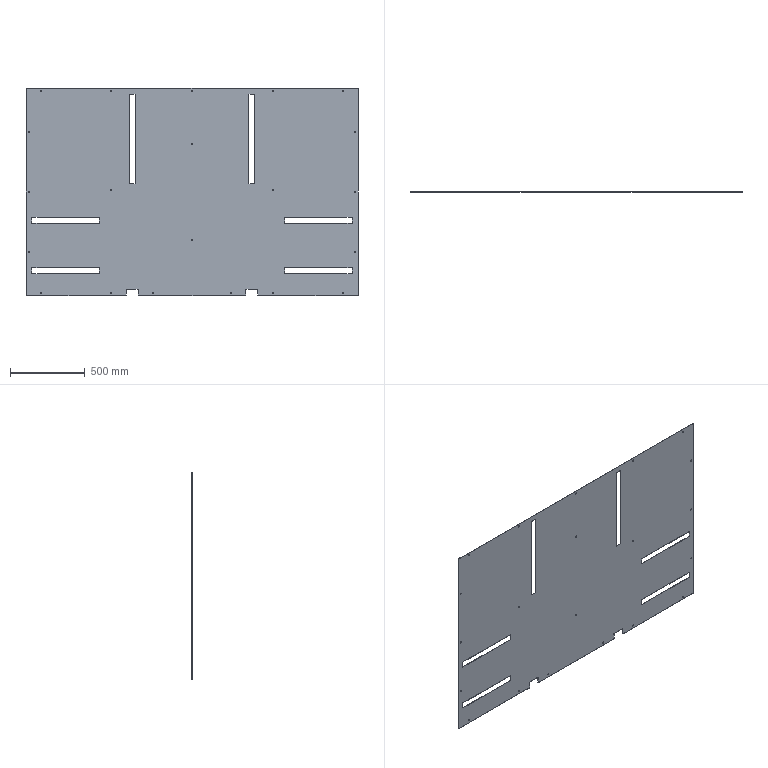Part | SolidWorks | features Fillet 2, ICE 2, FlatPattern 1, HoleWzd 1, SMBaseFlange 1, SheetMetal 1 | 1 solid | 88 faces | box 2220 x 2 x 1390 mm | volume 5915480 mm3 | cone 42 | plane 38 | cylinder 8 | commonest cylinder face diameters 9 x4 10 x4